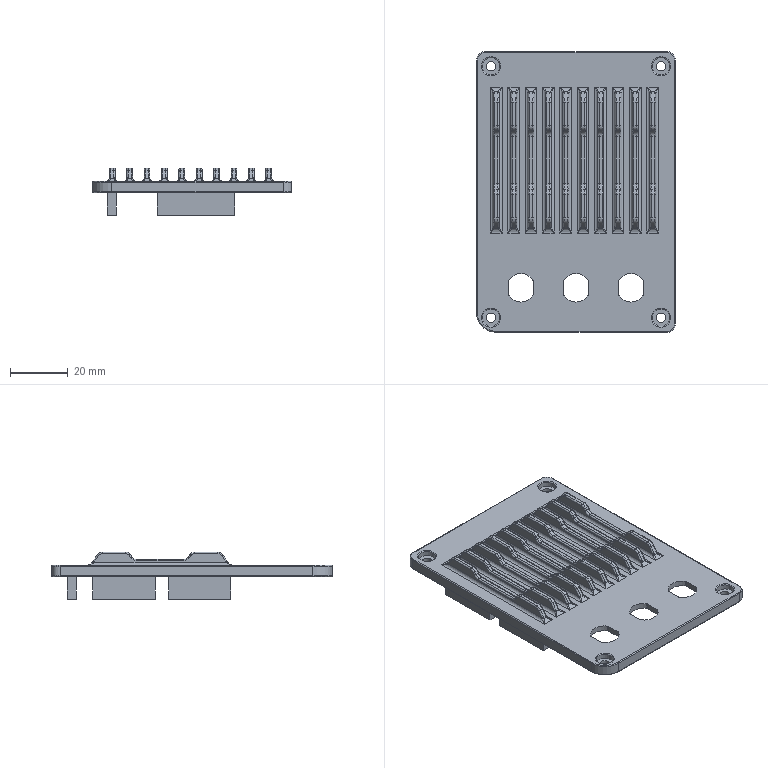NC program | NX | posted with a generic post | part box 68.665 x 96.782 x 16.5 mm
Lines 4798 to 5729 of 111885:
(CAVITY_MILL , TOOL : D8平刀)
N9510 T01 M6
N9512 G54
N9514 G17 G0 G90 X4. Y-42.331 S5500 M3
N9516 G43 Z20. H1
N9518 Z4.083
N9520 G94 G1 Z1.083 F3000.
N9522 Y-38.731
N9524 G3 X0. Y-34.731 R4.
N9526 G1 X-48.417
N9528 G2 X-48.788 Y-34.374 R0.401
N9530 G1 Y34.374
N9532 G2 X-48.417 Y34.731 R0.401
N9534 G1 X48.417
N9536 G2 X48.788 Y34.374 R0.401
N9538 G1 Y-34.374
N9540 G2 X48.417 Y-34.731 R0.401
N9542 G1 X0.
N9544 Y-28.331
N9546 X-42.388
N9548 Y28.331
N9550 X42.388
N9552 Y-28.331
N9554 X0.
N9556 Y-21.931
N9558 X-35.988
N9560 Y21.931
N9562 X35.988
N9564 Y-21.931
N9566 X0.
N9568 Y-15.531
N9570 X-29.588
N9572 Y15.531
N9574 X29.588
N9576 Y-15.531
N9578 X0.
N9580 Y-9.131
N9582 X-23.188
N9584 Y9.131
N9586 X23.188
N9588 Y-9.131
N9590 X0.
N9592 Y-2.731
N9594 X-16.788
N9596 Y2.731
N9598 X16.788
N9600 Y-2.731
N9602 X0.
N9604 G3 X-4. Y-6.731 R4.
N9606 G1 Z4.083
N9608 G0 X4. Y-42.331 Z3.667
N9610 G1 Z0.667
N9612 Y-38.731
N9614 G3 X0. Y-34.731 R4.
N9616 G1 X-48.417
N9618 G2 X-48.789 Y-34.373 R0.401
N9620 G1 X-48.79 Y-33.492
N9622 X-48.792 Y33.49
N9624 X-48.789 Y34.371
N9626 G2 X-48.417 Y34.731 R0.401
N9628 G1 X48.417
N9630 G2 X48.789 Y34.373 R0.401
N9632 G1 X48.79 Y33.492
N9634 X48.792 Y-33.49
N9636 X48.789 Y-34.371
N9638 G2 X48.417 Y-34.731 R0.401
N9640 G1 X0.
N9642 Y-28.331
N9644 X-42.39
N9646 X-42.391 Y28.331
N9648 X42.39
N9650 X42.391 Y-28.331
N9652 X0.
N9654 Y-21.931
N9656 X-35.991
N9658 Y21.931
N9660 X35.991
N9662 Y-21.931
N9664 X0.
N9666 Y-15.531
N9668 X-29.591
N9670 Y15.531
N9672 X29.591
N9674 Y-15.531
N9676 X0.
N9678 Y-9.131
N9680 X-23.191
N9682 Y9.131
N9684 X23.191
N9686 Y-9.131
N9688 X0.
N9690 Y-2.731
N9692 X-16.791
N9694 Y2.731
N9696 X16.791
N9698 Y-2.731
N9700 X0.
N9702 G3 X-4. Y-6.731 R4.
N9704 G1 Z3.667
N9706 G0 X4. Y-42.331 Z3.25
N9708 G1 Z0.25
N9710 Y-38.731
N9712 G3 X0. Y-34.731 R4.
N9714 G1 X-48.417
N9716 G2 X-48.789 Y-34.373 R0.401
N9718 G1 X-48.79 Y-33.492
N9720 X-48.792 Y33.49
N9722 X-48.789 Y34.371
N9724 G2 X-48.417 Y34.731 R0.401
N9726 G1 X48.417
N9728 G2 X48.789 Y34.373 R0.401
N9730 G1 X48.79 Y33.492
N9732 X48.792 Y-33.49
N9734 X48.789 Y-34.371
N9736 G2 X48.417 Y-34.731 R0.401
N9738 G1 X0.
N9740 Y-28.331
N9742 X-42.39
N9744 X-42.391 Y28.331
N9746 X42.39
N9748 X42.391 Y-28.331
N9750 X0.
N9752 Y-21.931
N9754 X-35.991
N9756 Y21.931
N9758 X35.991
N9760 Y-21.931
N9762 X0.
N9764 Y-15.531
N9766 X-29.591
N9768 Y15.531
N9770 X29.591
N9772 Y-15.531
N9774 X0.
N9776 Y-9.131
N9778 X-23.191
N9780 Y9.131
N9782 X23.191
N9784 Y-9.131
N9786 X0.
N9788 Y-2.731
N9790 X-16.791
N9792 Y2.731
N9794 X16.791
N9796 Y-2.731
N9798 X0.
N9800 G3 X-4. Y-6.731 R4.
N9802 G1 Z3.25
N9804 G0 X53.182 Y40.738 Z2.75
N9806 G1 Z-0.25
N9808 G3 X51.67 Y36.622 R4.
N9810 G2 X52.39 Y32.702 R43.098
N9812 G3 X56.39 Y29.243 R4.
N9814 G1 Z2.75
N9816 G0 X56.391 Y-30.267
N9818 G1 Z-0.25
N9820 G3 X52.391 Y-33.727 R4.
N9822 G2 X52.013 Y-36.027 R43.129
N9824 X48.475 Y-38.331 R4.001
N9826 G1 X44.874
N9828 G3 X46.384 Y-28.294 R36.729
N9830 G1 Y-26.619
N9832 G3 X46.292 Y-24.54 R37.077
N9834 X46.384 Y-22.246 R36.641
N9836 G1 Y-20.669
N9838 G3 X46.293 Y-18.546 R36.993
N9840 X46.384 Y-16.175 R36.536
N9842 G1 Y-14.719
N9844 G3 X46.293 Y-12.532 R36.91
N9846 X46.384 Y-10.238 R36.629
N9848 G1 Y-8.663
N9850 G3 X46.292 Y-6.535 R37.003
N9852 X46.384 Y-4.26 R36.663
N9854 G1 Y-2.658
N9856 G3 X46.293 Y-0.557 R37.011
N9858 X46.384 Y1.889 R36.445
N9860 G1 Y3.292
N9862 G3 X46.292 Y5.469 R36.928
N9864 X46.384 Y7.745 R36.651
N9866 G1 Y9.314
N9868 G3 X46.292 Y11.47 R36.964
N9870 X46.384 Y13.713 R36.703
N9872 G1 Y15.389
N9874 G3 X46.292 Y17.458 R37.092
N9876 X46.384 Y19.757 R36.636
N9878 G1 Y21.319
N9880 G3 X46.293 Y23.459 R36.973
N9882 X46.384 Y25.797 R36.578
N9884 G1 Y27.191
N9886 G3 X44.553 Y38.331 R36.698
N9888 G1 X37.738
N9890 G2 X39.984 Y27.161 R30.298
N9892 G1 Y25.822
N9894 G2 X39.873 Y23.458 R30.178
N9896 X39.984 Y21.271 R30.573
N9898 G1 Y19.788
N9900 G2 X39.872 Y17.456 R30.236
N9902 X39.984 Y15.331 R30.692
N9904 G1 Y13.75
N9906 G2 X39.872 Y11.47 R30.303
N9908 X39.984 Y9.266 R30.564
N9910 G1 Y7.777
N9912 G2 X39.872 Y5.468 R30.251
N9914 X39.984 Y3.248 R30.528
N9916 G1 Y1.901
N9918 G2 X39.874 Y-0.559 R30.045
N9920 X39.984 Y-2.709 R30.611
N9922 G1 Y-4.227
N9924 G2 X39.872 Y-6.536 R30.263
N9926 X39.984 Y-8.713 R30.603
N9928 G1 Y-10.208
N9930 G2 X39.873 Y-12.533 R30.229
N9932 X39.984 Y-14.762 R30.51
N9934 G1 Y-16.154
N9936 G2 X39.873 Y-18.548 R30.136
N9938 X39.984 Y-20.719 R30.593
N9940 G1 Y-22.215
N9942 G2 X39.872 Y-24.543 R30.241
N9944 X39.984 Y-26.676 R30.677
N9946 G1 Y-28.256
N9948 G2 X38.136 Y-38.331 R30.329
N9950 G1 X31.193
N9952 G3 X33.584 Y-28.214 R23.929
N9954 G1 Y-26.74
N9956 G3 X33.441 Y-24.545 R24.277
N9958 X33.584 Y-22.18 R23.841
N9960 G1 Y-20.774
N9962 G3 X33.443 Y-18.549 R24.193
N9964 X33.584 Y-16.13 R23.736
N9966 G1 Y-14.809
N9968 G3 X33.442 Y-12.533 R24.11
N9970 X33.584 Y-10.174 R23.829
N9972 G1 Y-8.77
N9974 G3 X33.441 Y-6.537 R24.203
N9976 X33.584 Y-4.19 R23.863
N9978 G1 Y-2.767
N9980 G3 X33.444 Y-0.56 R24.211
N9982 X33.584 Y1.915 R23.645
N9984 G1 Y3.199
N9986 G3 X33.442 Y5.468 R24.128
N9988 X33.584 Y7.813 R23.851
N9990 G1 Y9.214
N9992 G3 X33.441 Y11.47 R24.164
N9994 X33.584 Y13.791 R23.903
N9996 G1 Y15.266
N9998 G3 X33.441 Y17.454 R24.292
N10000 X33.584 Y19.822 R23.836
N10002 G1 Y21.217
N10004 G3 X33.442 Y23.457 R24.173
N10006 X33.584 Y25.85 R23.778
N10008 G1 Y27.128
N10010 G3 X30.663 Y38.331 R23.898
N10012 G1 X22.918
N10014 G2 X27.184 Y27.09 R17.498
N10016 G1 Y25.882
N10018 G2 X26.989 Y23.458 R17.378
N10020 X27.184 Y21.156 R17.773
N10022 G1 Y19.861
N10024 G2 X26.987 Y17.454 R17.436
N10026 X27.184 Y15.192 R17.892
N10028 G1 Y13.838
N10030 G2 X26.988 Y11.471 R17.503
N10032 X27.184 Y9.153 R17.764
N10034 G1 Y7.855
N10036 G2 X26.989 Y5.469 R17.451
N10038 X27.184 Y3.142 R17.728
N10040 G1 Y1.931
N10042 G2 X26.991 Y-0.559 R17.245
N10044 X27.184 Y-2.833 R17.811
N10046 G1 Y-4.148
N10048 G2 X26.988 Y-6.536 R17.463
N10050 X27.184 Y-8.835 R17.803
N10052 G1 Y-10.136
N10054 G2 X26.99 Y-12.532 R17.429
N10056 X27.184 Y-14.864 R17.71
N10058 G1 Y-16.103
N10060 G2 X26.99 Y-18.548 R17.336
N10062 X27.184 Y-20.838 R17.793
N10064 G1 Y-22.14
N10066 G2 X26.987 Y-24.544 R17.441
N10068 X27.184 Y-26.813 R17.877
N10070 G1 Y-28.166
N10072 G2 X23.744 Y-38.331 R17.529
N10074 G3 X23.301 Y-42.331 R4.
N10076 G1 Z2.75
N10078 G0 X-45.352
N10080 G1 Z-0.25
N10082 G3 X-45.812 Y-38.331 R4.
N10084 G2 X-49.231 Y-28.046 R17.181
N10086 G1 Y-26.823
N10088 G2 X-49.031 Y-24.526 R17.763
N10090 X-49.231 Y-22.221 R17.852
N10092 G1 Y-20.903
N10094 G2 X-49.035 Y-18.509 R17.515
N10096 X-49.231 Y-16.203 R17.79
N10098 G1 Y-14.891
N10100 G2 X-49.036 Y-12.517 R17.55
N10102 X-49.231 Y-10.186 R17.737
N10104 G1 Y-8.85
N10106 G2 X-49.032 Y-6.516 R17.675
N10108 X-49.231 Y-4.231 R17.883
N10110 G1 Y-2.903
N10112 G2 X-49.035 Y-0.504 R17.513
N10114 X-49.231 Y1.778 R17.855
N10116 G1 Y3.093
N10118 G2 X-49.036 Y5.488 R17.502
N10120 X-49.231 Y7.814 R17.736
N10122 G1 Y9.142
N10124 G2 X-49.034 Y11.477 R17.651
N10126 X-49.231 Y13.805 R17.764
N10128 G1 Y15.143
N10130 G2 X-49.033 Y17.484 R17.654
N10132 X-49.231 Y19.778 R17.853
N10134 G1 Y21.096
N10136 G2 X-49.036 Y23.487 R17.51
N10138 X-49.231 Y25.813 R17.738
N10140 G1 Y27.125
N10142 G2 X-44.953 Y38.331 R17.542
N10144 G3 X-44.224 Y42.331 R4.
N10146 G1 Z2.75
N10148 G0 X-20.955 Y-42.331
N10150 G1 Z-0.25
N10152 G2 X-18.37 Y-38.331 R4.
N10154 G3 X-11.139 Y-28.118 R11.163
N10156 G1 Y-26.897
N10158 G3 X-11.452 Y-24.538 R11.523
N10160 X-11.139 Y-22.096 R11.068
N10162 G1 Y-20.933
N10164 G3 X-11.447 Y-18.531 R11.313
N10166 X-11.139 Y-16.076 R10.969
N10168 G1 Y-14.925
N10170 G3 X-11.449 Y-12.527 R11.358
N10172 X-11.139 Y-10.094 R11.06
N10174 G1 Y-8.902
N10176 G3 X-11.453 Y-6.531 R11.493
N10178 X-11.139 Y-4.108 R11.13
N10180 G1 Y-2.929
N10182 G3 X-11.448 Y-0.53 R11.338
N10184 X-11.139 Y1.917 R11.006
N10186 G1 Y3.069
N10188 G3 X-11.447 Y5.47 R11.328
N10190 X-11.139 Y7.913 R11.083
N10192 G1 Y9.09
N10194 G3 X-11.453 Y11.476 R11.441
N10196 X-11.139 Y13.883 R11.177
N10198 G1 Y15.103
N10200 G3 X-11.451 Y17.457 R11.518
N10202 X-11.139 Y19.916 R11.009
N10204 G1 Y21.067
N10206 G3 X-11.446 Y23.468 R11.316
N10208 X-11.139 Y25.926 R10.962
N10210 G1 Y27.048
N10212 G3 X-18.827 Y37.445 R11.112
N10214 X-22.946 Y38.084 R13.742
N10216 G1 X-31.014
N10218 G3 X-35.295 Y37.393 R13.543
N10220 X-42.831 Y27.063 R11.142
N10222 G1 Y25.882
N10224 G3 X-42.521 Y23.484 R11.338
N10226 X-42.831 Y21.046 R11.11
N10228 G1 Y19.862
N10230 G3 X-42.516 Y17.481 R11.453
N10232 X-42.831 Y15.074 R11.254
N10234 G1 Y13.877
N10236 G3 X-42.518 Y11.474 R11.364
N10238 X-42.831 Y9.073 R11.251
N10240 G1 Y7.882
N10242 G3 X-42.522 Y5.484 R11.336
N10244 X-42.831 Y3.045 R11.102
N10246 G1 Y1.862
N10248 G3 X-42.519 Y-0.508 R11.455
N10250 X-42.831 Y-2.953 R11.113
N10252 G1 Y-4.143
N10254 G3 X-42.516 Y-6.519 R11.483
N10256 X-42.831 Y-8.923 R11.275
N10258 G1 Y-10.118
N10260 G3 X-42.521 Y-12.52 R11.337
N10262 X-42.831 Y-14.946 R11.15
N10264 G1 Y-16.127
N10266 G3 X-42.52 Y-18.513 R11.39
N10268 X-42.831 Y-20.953 R11.115
N10270 G1 Y-22.138
N10272 G3 X-42.515 Y-24.528 R11.452
N10274 X-42.831 Y-26.907 R11.363
N10276 G1 Y-28.046
N10278 G3 X-40.034 Y-35.29 R10.781
N10280 X-35.584 Y-38.331 R11.597
N10282 G2 X-33.021 Y-42.331 R4.
N10284 G1 Z2.75
N10286 G0 X10.936
N10288 G1 Z-0.25
N10290 G2 X13.535 Y-38.331 R4.
N10292 G3 X20.784 Y-28.106 R11.129
N10294 G1 Y-26.901
N10296 G3 X20.471 Y-24.538 R11.477
N10298 X20.784 Y-22.091 R11.041
N10300 G1 Y-20.916
N10302 G3 X20.475 Y-18.541 R11.393
N10304 X20.784 Y-16.07 R10.936
N10306 G1 Y-14.931
N10308 G3 X20.474 Y-12.527 R11.31
N10310 X20.784 Y-10.089 R11.029
N10312 G1 Y-8.914
N10314 G3 X20.472 Y-6.531 R11.403
N10316 X20.784 Y-4.096 R11.063
N10318 G1 Y-2.913
N10320 G3 X20.476 Y-0.551 R11.411
N10322 X20.784 Y1.95 R10.845
N10324 G1 Y3.073
N10326 G3 X20.473 Y5.474 R11.328
N10328 X20.784 Y7.906 R11.051
N10330 G1 Y9.079
N10332 G3 X20.472 Y11.475 R11.364
N10334 X20.784 Y13.896 R11.103
N10336 G1 Y15.101
N10338 G3 X20.471 Y17.46 R11.492
N10340 X20.784 Y19.91 R11.036
N10342 G1 Y21.081
N10344 G3 X20.474 Y23.464 R11.373
N10346 X20.784 Y25.921 R10.978
N10348 G1 Y27.043
N10350 G3 X13.048 Y37.457 R11.098
N10352 X8.978 Y38.084 R13.695
N10354 G1 X0.913
N10356 G3 X-3.519 Y37.338 R13.386
N10358 X-10.908 Y27.066 R11.143
N10360 G1 Y25.855
N10362 G3 X-10.594 Y23.489 R11.483
N10364 X-10.908 Y21.061 R11.183
N10366 G1 Y19.85
N10368 G3 X-10.594 Y17.494 R11.516
N10370 X-10.908 Y15.055 R11.151
N10372 G1 Y13.876
N10374 G3 X-10.593 Y11.465 R11.366
N10376 X-10.908 Y9.097 R11.379
N10378 G1 Y7.872
N10380 G3 X-10.595 Y5.477 R11.386
N10382 X-10.908 Y3.073 R11.248
N10384 G1 Y1.852
N10386 G3 X-10.595 Y-0.506 R11.503
N10388 X-10.908 Y-2.949 R11.131
N10390 G1 Y-4.129
N10392 G3 X-10.597 Y-6.513 R11.393
N10394 X-10.908 Y-8.949 R11.13
N10396 G1 Y-10.115
N10398 G3 X-10.595 Y-12.532 R11.313
N10400 X-10.908 Y-14.919 R11.292
N10402 G1 Y-16.147
N10404 G3 X-10.595 Y-18.508 R11.498
N10406 X-10.908 Y-20.945 R11.151
N10408 G1 Y-22.151
N10410 G3 X-10.594 Y-24.506 R11.523
N10412 X-10.908 Y-26.945 R11.153
N10414 G1 Y-28.109
N10416 G3 X-3.691 Y-38.331 R11.152
N10418 G1 X-1.434 Y-32.343
N10420 G2 X-4.508 Y-28.023 R4.752
N10422 G1 Y-27.023
N10424 G2 X-3.732 Y-24.535 R4.753
N10426 X-4.508 Y-22.023 R5.123
N10428 G1 Y-21.023
N10430 G2 X-3.732 Y-18.535 R4.751
N10432 X-4.508 Y-16.023 R5.098
N10434 G1 Y-15.023
N10436 G2 X-3.732 Y-12.535 R4.892
N10438 X-4.508 Y-10.023 R4.913
N10440 G1 Y-9.023
N10442 G2 X-3.732 Y-6.535 R4.73
N10444 X-4.508 Y-4.023 R4.993
N10446 G1 Y-3.023
N10448 G2 X-3.732 Y-0.535 R4.731
N10450 X-4.508 Y1.977 R5.103
N10452 G1 Y2.977
N10454 G2 X-3.732 Y5.465 R4.848
N10456 X-4.508 Y7.977 R4.986
N10458 G1 Y8.977
N10460 G2 X-3.732 Y11.465 R4.979
N10462 X-4.508 Y13.977 R4.966
N10464 G1 Y14.977
N10466 G2 X-3.732 Y17.465 R4.751
N10468 X-4.508 Y19.977 R5.116
N10470 G1 Y20.977
N10472 G2 X-3.732 Y23.465 R4.783
N10474 X-4.508 Y25.977 R5.083
N10476 G1 Y26.977
N10478 G2 X-1.385 Y31.304 R4.743
N10480 X0.906 Y31.684 R6.986
N10482 G1 X8.97
N10484 G2 X11.12 Y31.354 R7.295
N10486 X14.384 Y26.977 R4.698
N10488 G1 Y25.977
N10490 G2 X13.602 Y23.497 R4.578
N10492 X14.384 Y20.977 R4.973
N10494 G1 Y19.977
N10496 G2 X13.602 Y17.497 R4.636
N10498 X14.384 Y14.977 R5.092
N10500 G1 Y13.977
N10502 G2 X13.602 Y11.497 R4.703
N10504 X14.384 Y8.977 R4.964
N10506 G1 Y7.977
N10508 G2 X13.602 Y5.497 R4.651
N10510 X14.384 Y2.977 R4.928
N10512 G1 Y1.977
N10514 G2 X13.602 Y-0.503 R4.445
N10516 X14.384 Y-3.023 R5.011
N10518 G1 Y-4.023
N10520 G2 X13.602 Y-6.503 R4.663
N10522 X14.384 Y-9.023 R5.003
N10524 G1 Y-10.023
N10526 G2 X13.602 Y-12.503 R4.629
N10528 X14.384 Y-15.023 R4.91
N10530 G1 Y-16.023
N10532 G2 X13.602 Y-18.503 R4.536
N10534 X14.384 Y-21.023 R4.993
N10536 G1 Y-22.023
N10538 G2 X13.602 Y-24.503 R4.641
N10540 X14.384 Y-27.023 R5.077
N10542 G1 Y-28.023
N10544 G2 X11.082 Y-32.409 R4.729
N10546 X9.004 Y-32.712 R6.141
N10548 G1 X8.97 Y-32.73
N10550 X0.906
N10552 G2 X-0.693 Y-32.555 R10.193
N10554 X-1.434 Y-32.343 R4.752
N10556 G1 Z2.75
N10558 G0 X-26.985 Y38.084
N10560 G1 Z-0.25
N10562 Y31.684
N10564 X-22.953
N10566 G2 X-20.779 Y31.35 R7.342
N10568 X-17.539 Y26.977 R4.712
N10570 G1 Y25.977
N10572 G2 X-18.318 Y23.498 R4.562
N10574 X-17.539 Y20.977 R4.916
N10576 G1 Y19.977
N10578 G2 X-18.318 Y17.498 R4.609
N10580 X-17.539 Y14.977 R5.118
N10582 G1 Y13.977
N10584 G2 X-18.318 Y11.498 R4.777
N10586 X-17.539 Y8.977 R5.041
N10588 G1 Y7.977
N10590 G2 X-18.313 Y5.49 R4.683
N10592 X-17.539 Y2.977 R4.928
N10594 G1 Y1.977
N10596 G2 X-18.318 Y-0.502 R4.606
N10598 X-17.539 Y-3.023 R4.938
N10600 G1 Y-4.023
N10602 G2 X-18.318 Y-6.502 R4.73
N10604 X-17.539 Y-9.023 R5.093
N10606 G1 Y-10.023
N10608 G2 X-18.318 Y-12.502 R4.66
N10610 X-17.539 Y-15.023 R4.958
N10612 G1 Y-16.023
N10614 G2 X-18.318 Y-18.502 R4.569
N10616 X-17.539 Y-21.023 R4.913
N10618 G1 Y-22.023
N10620 G2 X-18.318 Y-24.502 R4.668
N10622 X-17.539 Y-27.023 R5.123
N10624 G1 Y-28.023
N10626 G2 X-20.759 Y-32.388 R4.763
N10628 G1 X-21.314 Y-32.54
N10630 X-21.472 Y-32.581
N10632 X-22.165 Y-32.688
N10634 X-22.857 Y-32.709
N10636 X-22.953 Y-32.73
N10638 X-31.017
N10640 X-31.169 Y-32.708
N10642 X-31.627 Y-32.692
N10644 G2 X-35.294 Y-30.99 R5.197
N10646 X-36.431 Y-28.046 R4.381
N10648 G1 Y-27.023
N10650 G2 X-35.656 Y-24.535 R4.963
N10652 X-36.431 Y-22.023 R5.052
N10654 G1 Y-21.023
N10656 G2 X-35.656 Y-18.535 R4.715
N10658 X-36.431 Y-16.023 R4.99
N10660 G1 Y-15.023
N10662 G2 X-35.656 Y-12.535 R4.75
N10664 X-36.431 Y-10.023 R4.937
N10666 G1 Y-9.023
N10668 G2 X-35.656 Y-6.535 R4.875
N10670 X-36.431 Y-4.023 R5.083
N10672 G1 Y-3.023
N10674 G2 X-35.656 Y-0.535 R4.713
N10676 X-36.431 Y1.977 R5.055
N10678 G1 Y2.977
N10680 G2 X-35.656 Y5.465 R4.702
N10682 X-36.431 Y7.977 R4.936
N10684 G1 Y8.977
N10686 G2 X-35.656 Y11.465 R4.851
N10688 X-36.431 Y13.977 R4.964
N10690 G1 Y14.977
N10692 G2 X-35.656 Y17.465 R4.854
N10694 X-36.431 Y19.977 R5.053
N10696 G1 Y20.977
N10698 G2 X-35.656 Y23.465 R4.71
N10700 X-36.431 Y25.977 R4.938
N10702 G1 Y26.977
N10704 G2 X-33.247 Y31.329 R4.742
N10706 X-31.017 Y31.684 R7.143
N10708 G1 X-26.985
N10710 G3 X-22.985 Y35.684 R4.
N10712 G1 Y42.331
N10714 Z2.75
N10716 G0 X46.398 Y-42.331 Z2.25
N10718 G1 Z-0.75
N10720 G2 X45.346 Y-38.331 R4.
N10722 G3 X46.841 Y-28.175 R36.763
N10724 G1 Y-26.813
N10726 G3 X46.751 Y-24.525 R36.867
N10728 X46.841 Y-22.219 R36.828
N10730 G1 Y-20.708
N10732 G3 X46.749 Y-18.526 R37.045
N10734 X46.841 Y-16.307 R36.974
N10736 G1 Y-14.751
N10738 G3 X46.749 Y-12.514 R36.971
N10740 X46.841 Y-10.375 R37.091
N10742 G1 Y-8.786
N10744 G3 X46.75 Y-6.519 R36.912
N10746 X46.841 Y-4.289 R36.944
N10748 G1 Y-2.835
N10750 G3 X46.751 Y-0.52 R36.831
N10752 X46.841 Y1.769 R36.847
N10754 G1 Y3.278
N10756 G3 X46.749 Y5.477 R37.02
N10758 X46.841 Y7.674 R37.005
N10760 G1 Y9.227
N10762 G3 X46.75 Y11.472 R36.935
N10764 X46.841 Y13.765 R36.855
N10766 G1 Y15.172
N10768 G3 X46.751 Y17.479 R36.843
N10770 X46.841 Y19.772 R36.842
N10772 G1 Y21.275
N10774 G3 X46.749 Y23.477 R37.015
N10776 X46.841 Y25.683 R36.991
N10778 G1 Y27.147
N10780 G3 X45.02 Y38.331 R36.782
N10782 G1 X38.209
N10784 G2 X40.441 Y27.124 R30.382
N10786 G1 Y25.724
N10788 G2 X40.329 Y23.477 R30.591
N10790 X40.441 Y21.233 R30.615
N10792 G1 Y19.801
N10794 G2 X40.331 Y17.479 R30.442
N10796 X40.441 Y15.145 R30.443
N10798 G1 Y13.794
N10800 G2 X40.331 Y11.472 R30.455
N10802 X40.441 Y9.192 R30.535
N10804 G1 Y7.717
N10806 G2 X40.329 Y5.477 R30.605
N10808 X40.441 Y3.236 R30.62
N10810 G1 Y1.798
N10812 G2 X40.331 Y-0.52 R30.447
N10814 X40.441 Y-2.862 R30.431
N10816 G1 Y-4.252
N10818 G2 X40.33 Y-6.519 R30.544
N10820 X40.441 Y-8.82 R30.512
N10822 G1 Y-10.325
N10824 G2 X40.329 Y-12.513 R30.691
N10826 X40.441 Y-14.789 R30.571
N10828 G1 Y-16.267
N10830 G2 X40.329 Y-18.527 R30.574
N10832 X40.441 Y-20.752 R30.645
N10834 G1 Y-22.192
N10836 G2 X40.331 Y-24.525 R30.428
N10838 X40.441 Y-26.843 R30.467
N10840 G1 Y-28.154
N10842 G2 X38.613 Y-38.331 R30.363
N10844 G1 X31.678
N10846 G3 X34.041 Y-28.13 R23.963
N10848 G1 Y-26.875
N10850 G3 X33.902 Y-24.525 R24.067
N10852 X34.041 Y-22.161 R24.028
N10854 G1 Y-20.802
N10856 G3 X33.899 Y-18.527 R24.245
N10858 X34.041 Y-16.223 R24.174
N10860 G1 Y-14.832
N10862 G3 X33.898 Y-12.512 R24.171
N10864 X34.041 Y-10.27 R24.291
N10866 G1 Y-8.857
N10868 G3 X33.9 Y-6.518 R24.112
N10870 X34.041 Y-4.21 R24.144
N10872 G1 Y-2.891
N10874 G3 X33.902 Y-0.52 R24.031
N10876 X34.041 Y1.831 R24.047
N10878 G1 Y3.188
N10880 G3 X33.898 Y5.478 R24.22
N10882 X34.041 Y7.764 R24.205
N10884 G1 Y9.153
N10886 G3 X33.901 Y11.472 R24.135
N10888 X34.041 Y13.828 R24.055
N10890 G1 Y15.114
N10892 G3 X33.902 Y17.479 R24.043
N10894 X34.041 Y19.833 R24.042
N10896 G1 Y21.186
N10898 G3 X33.899 Y23.477 R24.215
N10900 X34.041 Y25.77 R24.191
N10902 G1 Y27.097
N10904 G3 X31.141 Y38.331 R23.982
N10906 G1 X23.417
N10908 G2 X27.641 Y27.067 R17.582
N10910 G1 Y25.823
N10912 G2 X27.446 Y23.477 R17.791
N10914 X27.641 Y21.133 R17.815
N10916 G1 Y19.87
N10918 G2 X27.45 Y17.479 R17.642
N10920 X27.641 Y15.079 R17.643
N10922 G1 Y13.866
N10924 G2 X27.449 Y11.472 R17.655
N10926 X27.641 Y9.108 R17.735
N10928 G1 Y7.819
N10930 G2 X27.446 Y5.478 R17.805
N10932 X27.641 Y3.134 R17.82
N10934 G1 Y1.868
N10936 G2 X27.45 Y-0.519 R17.647
N10938 X27.641 Y-2.925 R17.631
N10940 G1 Y-4.162
N10942 G2 X27.448 Y-6.518 R17.744
N10944 X27.641 Y-8.899 R17.712
N10946 G1 Y-10.206
N10948 G2 X27.445 Y-12.511 R17.891
N10950 X27.641 Y-14.881 R17.771
N10952 G1 Y-16.171
N10954 G2 X27.446 Y-18.527 R17.774
N10956 X27.641 Y-20.859 R17.845
N10958 G1 Y-22.126
N10960 G2 X27.45 Y-24.524 R17.628
N10962 X27.641 Y-26.913 R17.667
N10964 G1 Y-28.103
N10966 G2 X24.247 Y-38.331 R17.563
N10968 G3 X23.824 Y-42.331 R4.
N10970 G1 Z2.25
N10972 G0 X-45.871
N10974 G1 Z-0.75
N10976 G3 X-46.294 Y-38.331 R4.
N10978 G2 X-49.688 Y-28.107 R17.572
N10980 G1 Y-26.968
N10982 G2 X-49.499 Y-24.513 R17.43
N10984 X-49.688 Y-22.119 R17.626
N10986 G1 Y-20.95
N10988 G2 X-49.5 Y-18.526 R17.481
N10990 X-49.688 Y-16.092 R17.544
N10992 G1 Y-15.012
N10994 G2 X-49.5 Y-12.493 R17.306
N10996 X-49.688 Y-10.14 R17.691
N10998 G1 Y-8.982
N11000 G2 X-49.499 Y-6.504 R17.39
N11002 X-49.688 Y-4.135 R17.674
N11004 G1 Y-2.955
N11006 G2 X-49.499 Y-0.521 R17.468
N11008 X-49.688 Y1.895 R17.581
N11010 G1 Y3.024
N11012 G2 X-49.5 Y5.489 R17.408
N11014 X-49.688 Y7.884 R17.606
N11016 G1 Y9.021
N11018 G2 X-49.499 Y11.498 R17.399
N11020 X-49.688 Y13.853 R17.712
N11022 G1 Y15.037
N11024 G2 X-49.499 Y17.484 R17.445
N11026 X-49.688 Y19.885 R17.613
N11028 G1 Y21.042
N11030 G2 X-49.499 Y23.479 R17.46
N11032 X-49.688 Y25.896 R17.578
N11034 G1 Y27.044
N11036 G2 X-45.47 Y38.331 R17.541
N11038 G3 X-44.761 Y42.331 R4.
N11040 G1 Z2.25
N11042 G0 X-20.226 Y-42.331
N11044 G1 Z-0.75
N11046 G2 X-17.719 Y-38.331 R4.
N11048 G3 X-11.024 Y-30.692 R11.184
N11050 X-6.182 Y-37.381 R11.164
N11052 X-4.308 Y-38.331 R11.785
N11054 G2 X-1.802 Y-42.331 R4.
N11056 G1 Z2.25
N11058 G0 X11.674
N11060 G1 Z-0.75
N11062 G2 X14.19 Y-38.331 R4.
N11064 G3 X21.241 Y-28.07 R11.163
N11066 G1 Y-26.959
N11068 G3 X20.939 Y-24.524 R11.267
N11070 X21.241 Y-22.083 R11.228
N11072 G1 Y-20.928
N11074 G3 X20.933 Y-18.526 R11.445
N11076 X21.241 Y-16.109 R11.374
N11078 G1 Y-14.941
N11080 G3 X20.932 Y-12.512 R11.371
N11082 X21.241 Y-10.129 R11.491
N11084 G1 Y-8.951
N11086 G3 X20.936 Y-6.518 R11.312
N11088 X21.241 Y-4.104 R11.344
N11090 G1 Y-2.966
N11092 G3 X20.939 Y-0.52 R11.231
N11094 X21.241 Y1.914 R11.247
N11096 G1 Y3.068
N11098 G3 X20.933 Y5.478 R11.42
N11100 X21.241 Y7.885 R11.405
N11102 G1 Y9.053
N11104 G3 X20.937 Y11.473 R11.335
N11106 X21.241 Y13.912 R11.255
N11108 G1 Y15.036
N11110 G3 X20.939 Y17.479 R11.243
N11112 X21.241 Y19.915 R11.242
N11114 G1 Y21.067
N11116 G3 X20.933 Y23.477 R11.415
N11118 X21.241 Y25.888 R11.391
N11120 G1 Y27.029
N11122 G3 X15.646 Y36.586 R11.182
N11124 X9.648 Y38.127 R11.845
N11126 G1 X0.086
N11128 G3 X-4.603 Y37.161 R11.764
N11130 X-11.025 Y29.655 R11.125
N11132 G1 X-8.965 Y26.227
N11134 Y25.977
N11136 G3 X-8.581 Y23.484 R8.892
N11138 X-8.965 Y20.977 R8.694
N11140 G1 Y19.977
N11142 G3 X-8.578 Y17.48 R8.924
N11144 X-8.965 Y14.977 R8.78
N11146 G1 Y13.977
N11148 G3 X-8.581 Y11.489 R8.931
N11150 X-8.965 Y8.977 R8.662
N11152 G1 Y7.977
N11154 G3 X-8.582 Y5.48 R8.83
N11156 X-8.965 Y2.977 R8.709
N11158 G1 Y1.977
N11160 G3 X-8.579 Y-0.519 R8.922
N11162 X-8.965 Y-3.023 R8.762
N11164 G1 Y-4.023
N11166 G3 X-8.579 Y-6.518 R8.934
N11168 X-8.965 Y-9.023 R8.758
N11170 G1 Y-10.023
N11172 G3 X-8.582 Y-12.521 R8.832
N11174 X-8.965 Y-15.023 R8.707
N11176 G1 Y-16.023
N11178 G3 X-8.581 Y-18.515 R8.887
N11180 X-8.965 Y-21.023 R8.679
N11182 G1 Y-22.023
N11184 G3 X-8.578 Y-24.521 R8.914
N11186 X-8.965 Y-27.023 R8.789
N11188 G1 Y-27.263
N11190 G3 X-13.082 Y-27.262 R4.
N11192 G1 Y-27.023
N11194 G3 X-13.462 Y-24.54 R8.678
N11196 X-13.186 Y-23.197 R7.77
N11198 G1 X-13.172 Y-23.053
N11200 X-13.147 Y-22.744
N11202 G3 X-13.082 Y-22.023 R4.
N11204 G1 Y-21.023
N11206 G3 X-13.468 Y-18.527 R8.74
N11208 X-13.082 Y-16.023 R8.58
N11210 G1 Y-15.023
N11212 G3 X-13.469 Y-12.521 R8.705
N11214 X-13.082 Y-10.023 R8.635
N11216 G1 Y-9.023
N11218 G3 X-13.144 Y-8.319 R4.
N11220 G1 X-13.162 Y-8.104
N11222 G3 X-13.455 Y-6.521 R7.802
N11224 X-13.206 Y-5.337 R7.671
N11226 G1 X-13.191 Y-5.206
N11228 X-13.146 Y-4.736
N11230 G3 X-13.082 Y-4.023 R4.
N11232 G1 Y-3.023
N11234 G3 X-13.47 Y-0.53 R8.794
N11236 X-13.082 Y1.977 R8.59
N11238 G1 Y2.977
N11240 G3 X-13.469 Y5.476 R8.734
N11242 X-13.082 Y7.977 R8.616
N11244 G1 Y8.977
N11246 G3 X-13.467 Y11.49 R8.597
N11248 X-13.086 Y13.785 R10.005
N11250 G1 X-13.082 Y13.977
N11252 Y14.977
N11254 G3 X-13.466 Y17.474 R8.676
N11256 X-13.082 Y19.977 R8.531
N11258 G1 Y20.977
N11260 G3 X-13.469 Y23.472 R8.754
N11262 X-13.082 Y25.977 R8.586
N11264 G1 Y26.224
N11266 G3 X-8.965 Y26.227 R4.
N11268 G1 X-11.025 Y29.655
N11270 G3 X-14.525 Y35.349 R11.207
N11272 X-22.204 Y38.127 R11.672
N11274 G1 X-31.891
N11276 G3 X-36.968 Y36.948 R11.524
N11278 G1 X-37.573 Y36.651
N11280 G3 X-43.288 Y27.017 R11.141
N11282 G1 Y25.93
N11284 G3 X-42.989 Y23.477 R11.178
N11286 X-43.288 Y21.015 R11.06
N11288 G1 Y19.923
N11290 G3 X-42.988 Y17.481 R11.213
N11292 X-43.288 Y15.012 R11.045
N11294 G1 Y13.905
N11296 G3 X-42.987 Y11.493 R11.312
N11298 X-43.288 Y9.003 R10.999
N11300 G1 Y7.923
N11302 G3 X-42.989 Y5.485 R11.206
N11304 X-43.288 Y3.005 R11.008
N11306 G1 Y1.929
N11308 G3 X-42.988 Y-0.523 R11.181
N11310 X-43.288 Y-2.983 R11.068
N11312 G1 Y-4.088
N11314 G3 X-42.988 Y-6.509 R11.274
N11316 X-43.288 Y-8.999 R10.99
N11318 G1 Y-10.091
N11320 G3 X-42.99 Y-12.5 R11.291
N11322 X-43.288 Y-15.017 R10.906
N11324 G1 Y-16.063
N11326 G3 X-42.989 Y-18.528 R11.144
N11328 X-43.288 Y-20.981 R11.081
N11330 G1 Y-22.079
N11332 G3 X-42.988 Y-24.516 R11.226
N11334 X-43.288 Y-26.991 R11.03
N11336 G1 Y-28.072
N11338 G3 X-37.959 Y-37.473 R11.172
N11340 X-36.229 Y-38.331 R11.847
N11342 G1 X-33.86 Y-32.386
N11344 G2 X-34.632 Y-32.005 R5.447
N11346 X-36.888 Y-28.023 R4.772
N11348 G1 Y-27.023
N11350 G2 X-36.131 Y-24.533 R4.63
N11352 X-36.888 Y-22.023 R4.826
N11354 G1 Y-21.023
N11356 G2 X-36.131 Y-18.533 R4.681
N11358 X-36.888 Y-16.023 R4.744
N11360 G1 Y-15.023
N11362 G2 X-36.131 Y-12.533 R4.506
N11364 X-36.888 Y-10.023 R4.891
N11366 G1 Y-9.023